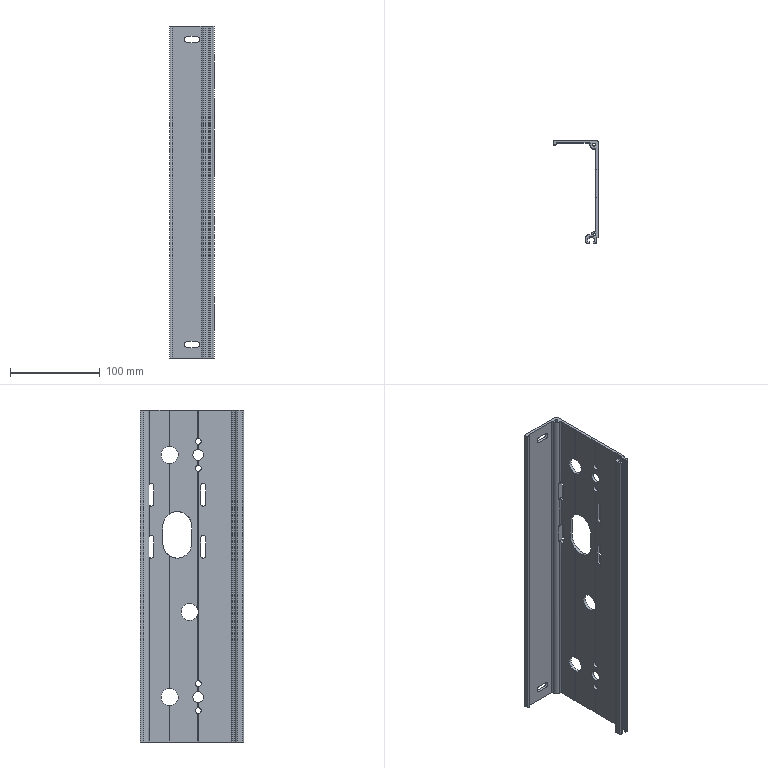Part | STEP file | 601-12-0009 | 1 solid | 148 faces | box 50.06 x 115 x 370 mm | volume 200376 mm3 | cylinder 71 | plane 67 | cone 10 | commonest cylinder face diameters 5.5 x12 3.3 x10 6.5 x8 0.4 x6 7 x6 19 x6